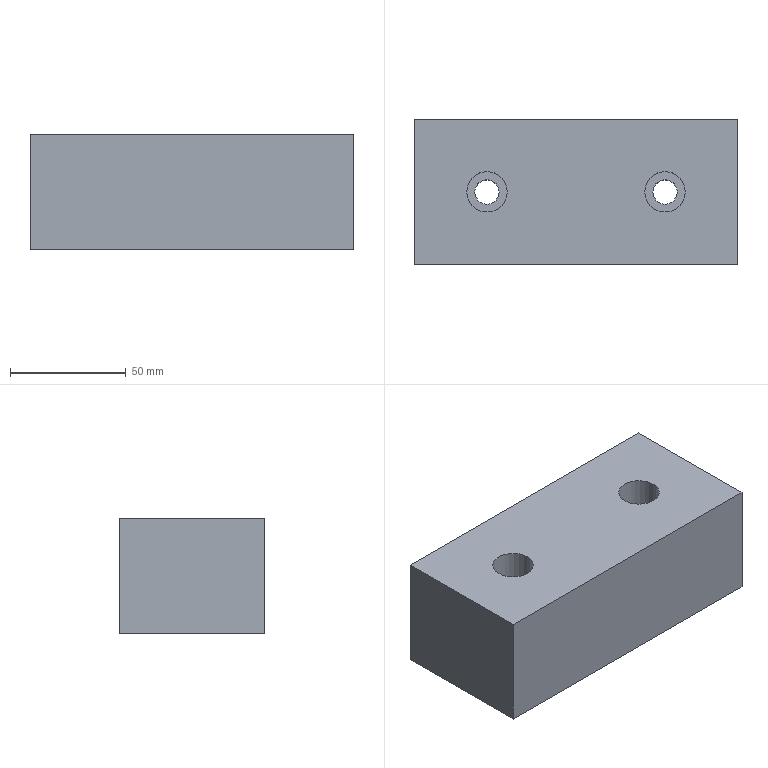Part | NX | features MAIN_BODY 2 | 1 solid | 12 faces | box 140 x 63 x 50 mm | volume 423105 mm3 | plane 8 | cylinder 4 | commonest cylinder face diameters 10.5 x2 17.5 x2
STEP:
#1=CARTESIAN_POINT('',(1506.25,487.5,70.));
#2=VERTEX_POINT('',#1);
#3=CARTESIAN_POINT('',(1511.5,487.5,70.));
#4=DIRECTION('',(0.,0.,-1.));
#5=DIRECTION('',(-1.,0.,0.));
#6=AXIS2_PLACEMENT_3D('',#3,#4,#5);
#7=CIRCLE('',#6,5.25);
#8=EDGE_CURVE('',#2,#2,#7,.F.);
#9=ORIENTED_EDGE('',*,*,#8,.F.);
#10=EDGE_LOOP('',(#9));
#11=FACE_BOUND('',#10,.T.);
#12=CARTESIAN_POINT('',(1506.25,487.5,90.));
#13=VERTEX_POINT('',#12);
#14=CARTESIAN_POINT('',(1511.5,487.5,90.));
#15=DIRECTION('',(0.,0.,-1.));
#16=DIRECTION('',(-1.,0.,0.));
#17=AXIS2_PLACEMENT_3D('',#14,#15,#16);
#18=CIRCLE('',#17,5.25);
#19=EDGE_CURVE('',#13,#13,#18,.F.);
#20=ORIENTED_EDGE('',*,*,#19,.T.);
#21=EDGE_LOOP('',(#20));
#22=FACE_BOUND('',#21,.T.);
#23=CARTESIAN_POINT('',(1511.5,487.5,90.));
#24=DIRECTION('',(0.,0.,-1.));
#25=DIRECTION('',(-1.,0.,0.));
#26=AXIS2_PLACEMENT_3D('',#23,#24,#25);
#27=CYLINDRICAL_SURFACE('',#26,5.25);
#28=ADVANCED_FACE('',(#11,#22),#27,.F.);
#29=CARTESIAN_POINT('',(1593.75,487.5,70.));
#30=VERTEX_POINT('',#29);
#31=CARTESIAN_POINT('',(1588.5,487.5,70.));
#32=DIRECTION('',(0.,0.,1.));
#33=DIRECTION('',(1.,0.,0.));
#34=AXIS2_PLACEMENT_3D('',#31,#32,#33);
#35=CIRCLE('',#34,5.25);
#36=EDGE_CURVE('',#30,#30,#35,.F.);
#37=ORIENTED_EDGE('',*,*,#36,.T.);
#38=EDGE_LOOP('',(#37));
#39=FACE_BOUND('',#38,.T.);
#40=CARTESIAN_POINT('',(1593.75,487.5,90.));
#41=VERTEX_POINT('',#40);
#42=CARTESIAN_POINT('',(1588.5,487.5,90.));
#43=DIRECTION('',(0.,0.,1.));
#44=DIRECTION('',(1.,0.,0.));
#45=AXIS2_PLACEMENT_3D('',#42,#43,#44);
#46=CIRCLE('',#45,5.25);
#47=EDGE_CURVE('',#41,#41,#46,.F.);
#48=ORIENTED_EDGE('',*,*,#47,.F.);
#49=EDGE_LOOP('',(#48));
#50=FACE_BOUND('',#49,.T.);
#51=CARTESIAN_POINT('',(1588.5,487.5,90.));
#52=DIRECTION('',(0.,0.,-1.));
#53=DIRECTION('',(1.,0.,0.));
#54=AXIS2_PLACEMENT_3D('',#51,#52,#53);
#55=CYLINDRICAL_SURFACE('',#54,5.25);
#56=ADVANCED_FACE('',(#39,#50),#55,.F.);
#57=ORIENTED_EDGE('',*,*,#47,.T.);
#58=EDGE_LOOP('',(#57));
#59=FACE_BOUND('',#58,.T.);
#60=CARTESIAN_POINT('',(1597.25,487.5,90.));
#61=VERTEX_POINT('',#60);
#62=CARTESIAN_POINT('',(1588.5,487.5,90.));
#63=DIRECTION('',(0.,0.,-1.));
#64=DIRECTION('',(1.,0.,0.));
#65=AXIS2_PLACEMENT_3D('',#62,#63,#64);
#66=CIRCLE('',#65,8.75);
#67=EDGE_CURVE('',#61,#61,#66,.T.);
#68=ORIENTED_EDGE('',*,*,#67,.F.);
#69=EDGE_LOOP('',(#68));
#70=FACE_BOUND('',#69,.T.);
#71=CARTESIAN_POINT('',(1588.5,487.5,90.));
#72=DIRECTION('',(0.,0.,-1.));
#73=DIRECTION('',(1.,0.,0.));
#74=AXIS2_PLACEMENT_3D('',#71,#72,#73);
#75=PLANE('',#74);
#76=ADVANCED_FACE('',(#59,#70),#75,.F.);
#77=ORIENTED_EDGE('',*,*,#67,.T.);
#78=EDGE_LOOP('',(#77));
#79=FACE_BOUND('',#78,.T.);
#80=CARTESIAN_POINT('',(1597.25,487.5,120.));
#81=VERTEX_POINT('',#80);
#82=CARTESIAN_POINT('',(1588.5,487.5,120.));
#83=DIRECTION('',(0.,0.,1.));
#84=DIRECTION('',(1.,0.,0.));
#85=AXIS2_PLACEMENT_3D('',#82,#83,#84);
#86=CIRCLE('',#85,8.75);
#87=EDGE_CURVE('',#81,#81,#86,.F.);
#88=ORIENTED_EDGE('',*,*,#87,.F.);
#89=EDGE_LOOP('',(#88));
#90=FACE_BOUND('',#89,.T.);
#91=CARTESIAN_POINT('',(1588.5,487.5,70.));
#92=DIRECTION('',(0.,0.,1.));
#93=DIRECTION('',(1.,0.,0.));
#94=AXIS2_PLACEMENT_3D('',#91,#92,#93);
#95=CYLINDRICAL_SURFACE('',#94,8.75);
#96=ADVANCED_FACE('',(#79,#90),#95,.F.);
#97=ORIENTED_EDGE('',*,*,#36,.F.);
#98=EDGE_LOOP('',(#97));
#99=FACE_BOUND('',#98,.T.);
#100=CARTESIAN_POINT('',(1620.,456.,70.));
#101=VERTEX_POINT('',#100);
#102=CARTESIAN_POINT('',(1620.,519.,70.));
#103=VERTEX_POINT('',#102);
#104=CARTESIAN_POINT('',(1620.,469.,70.));
#105=DIRECTION('',(0.,1.,0.));
#106=VECTOR('',#105,1000.);
#107=LINE('',#104,#106);
#108=EDGE_CURVE('',#101,#103,#107,.T.);
#109=ORIENTED_EDGE('',*,*,#108,.F.);
#110=CARTESIAN_POINT('',(1480.,456.,70.));
#111=VERTEX_POINT('',#110);
#112=CARTESIAN_POINT('',(1343.352,456.,70.));
#113=DIRECTION('',(1.,0.,0.));
#114=VECTOR('',#113,1000.);
#115=LINE('',#112,#114);
#116=EDGE_CURVE('',#111,#101,#115,.T.);
#117=ORIENTED_EDGE('',*,*,#116,.F.);
#118=CARTESIAN_POINT('',(1480.,519.,70.));
#119=VERTEX_POINT('',#118);
#120=CARTESIAN_POINT('',(1480.,469.,70.));
#121=DIRECTION('',(0.,1.,0.));
#122=VECTOR('',#121,1000.);
#123=LINE('',#120,#122);
#124=EDGE_CURVE('',#111,#119,#123,.T.);
#125=ORIENTED_EDGE('',*,*,#124,.T.);
#126=CARTESIAN_POINT('',(1343.352,519.,70.));
#127=DIRECTION('',(1.,0.,0.));
#128=VECTOR('',#127,1000.);
#129=LINE('',#126,#128);
#130=EDGE_CURVE('',#119,#103,#129,.T.);
#131=ORIENTED_EDGE('',*,*,#130,.T.);
#132=EDGE_LOOP('',(#109,#117,#125,#131));
#133=FACE_BOUND('',#132,.T.);
#134=ORIENTED_EDGE('',*,*,#8,.T.);
#135=EDGE_LOOP('',(#134));
#136=FACE_BOUND('',#135,.T.);
#137=CARTESIAN_POINT('',(1343.352,469.,70.));
#138=DIRECTION('',(0.,0.,-1.));
#139=DIRECTION('',(-1.,0.,0.));
#140=AXIS2_PLACEMENT_3D('',#137,#138,#139);
#141=PLANE('',#140);
#142=ADVANCED_FACE('',(#99,#133,#136),#141,.T.);
#143=ORIENTED_EDGE('',*,*,#19,.F.);
#144=EDGE_LOOP('',(#143));
#145=FACE_BOUND('',#144,.T.);
#146=CARTESIAN_POINT('',(1502.75,487.5,90.));
#147=VERTEX_POINT('',#146);
#148=CARTESIAN_POINT('',(1511.5,487.5,90.));
#149=DIRECTION('',(0.,0.,1.));
#150=DIRECTION('',(-1.,0.,0.));
#151=AXIS2_PLACEMENT_3D('',#148,#149,#150);
#152=CIRCLE('',#151,8.75);
#153=EDGE_CURVE('',#147,#147,#152,.T.);
#154=ORIENTED_EDGE('',*,*,#153,.T.);
#155=EDGE_LOOP('',(#154));
#156=FACE_BOUND('',#155,.T.);
#157=CARTESIAN_POINT('',(1511.5,487.5,90.));
#158=DIRECTION('',(0.,0.,-1.));
#159=DIRECTION('',(-1.,0.,0.));
#160=AXIS2_PLACEMENT_3D('',#157,#158,#159);
#161=PLANE('',#160);
#162=ADVANCED_FACE('',(#145,#156),#161,.F.);
#163=CARTESIAN_POINT('',(1620.,519.,120.));
#164=VERTEX_POINT('',#163);
#165=CARTESIAN_POINT('',(1620.,456.,120.));
#166=VERTEX_POINT('',#165);
#167=CARTESIAN_POINT('',(1620.,469.,120.));
#168=DIRECTION('',(0.,-1.,0.));
#169=VECTOR('',#168,1000.);
#170=LINE('',#167,#169);
#171=EDGE_CURVE('',#164,#166,#170,.T.);
#172=ORIENTED_EDGE('',*,*,#171,.T.);
#173=CARTESIAN_POINT('',(1620.,456.,228.412));
#174=DIRECTION('',(0.,0.,1.));
#175=VECTOR('',#174,1000.);
#176=LINE('',#173,#175);
#177=EDGE_CURVE('',#101,#166,#176,.T.);
#178=ORIENTED_EDGE('',*,*,#177,.F.);
#179=ORIENTED_EDGE('',*,*,#108,.T.);
#180=CARTESIAN_POINT('',(1620.,519.,70.));
#181=DIRECTION('',(0.,0.,1.));
#182=VECTOR('',#181,1000.);
#183=LINE('',#180,#182);
#184=EDGE_CURVE('',#103,#164,#183,.T.);
#185=ORIENTED_EDGE('',*,*,#184,.T.);
#186=EDGE_LOOP('',(#172,#178,#179,#185));
#187=FACE_BOUND('',#186,.T.);
#188=CARTESIAN_POINT('',(1620.,469.,70.));
#189=DIRECTION('',(1.,0.,0.));
#190=DIRECTION('',(0.,-1.,0.));
#191=AXIS2_PLACEMENT_3D('',#188,#189,#190);
#192=PLANE('',#191);
#193=ADVANCED_FACE('',(#187),#192,.T.);
#194=CARTESIAN_POINT('',(1480.,519.,120.));
#195=VERTEX_POINT('',#194);
#196=CARTESIAN_POINT('',(1480.,456.,120.));
#197=VERTEX_POINT('',#196);
#198=CARTESIAN_POINT('',(1480.,469.,120.));
#199=DIRECTION('',(0.,-1.,0.));
#200=VECTOR('',#199,1000.);
#201=LINE('',#198,#200);
#202=EDGE_CURVE('',#195,#197,#201,.T.);
#203=ORIENTED_EDGE('',*,*,#202,.F.);
#204=CARTESIAN_POINT('',(1480.,519.,70.));
#205=DIRECTION('',(0.,0.,1.));
#206=VECTOR('',#205,1000.);
#207=LINE('',#204,#206);
#208=EDGE_CURVE('',#119,#195,#207,.T.);
#209=ORIENTED_EDGE('',*,*,#208,.F.);
#210=ORIENTED_EDGE('',*,*,#124,.F.);
#211=CARTESIAN_POINT('',(1480.,456.,228.412));
#212=DIRECTION('',(0.,0.,1.));
#213=VECTOR('',#212,1000.);
#214=LINE('',#211,#213);
#215=EDGE_CURVE('',#111,#197,#214,.T.);
#216=ORIENTED_EDGE('',*,*,#215,.T.);
#217=EDGE_LOOP('',(#203,#209,#210,#216));
#218=FACE_BOUND('',#217,.T.);
#219=CARTESIAN_POINT('',(1480.,469.,70.));
#220=DIRECTION('',(-1.,0.,0.));
#221=DIRECTION('',(0.,-1.,0.));
#222=AXIS2_PLACEMENT_3D('',#219,#220,#221);
#223=PLANE('',#222);
#224=ADVANCED_FACE('',(#218),#223,.T.);
#225=ORIENTED_EDGE('',*,*,#171,.F.);
#226=CARTESIAN_POINT('',(1343.352,519.,120.));
#227=DIRECTION('',(1.,0.,0.));
#228=VECTOR('',#227,1000.);
#229=LINE('',#226,#228);
#230=EDGE_CURVE('',#195,#164,#229,.T.);
#231=ORIENTED_EDGE('',*,*,#230,.F.);
#232=ORIENTED_EDGE('',*,*,#202,.T.);
#233=CARTESIAN_POINT('',(1343.352,456.,120.));
#234=DIRECTION('',(1.,0.,0.));
#235=VECTOR('',#234,1000.);
#236=LINE('',#233,#235);
#237=EDGE_CURVE('',#197,#166,#236,.T.);
#238=ORIENTED_EDGE('',*,*,#237,.T.);
#239=EDGE_LOOP('',(#225,#231,#232,#238));
#240=FACE_BOUND('',#239,.T.);
#241=CARTESIAN_POINT('',(1502.75,487.5,120.));
#242=VERTEX_POINT('',#241);
#243=CARTESIAN_POINT('',(1511.5,487.5,120.));
#244=DIRECTION('',(0.,0.,-1.));
#245=DIRECTION('',(-1.,0.,0.));
#246=AXIS2_PLACEMENT_3D('',#243,#244,#245);
#247=CIRCLE('',#246,8.75);
#248=EDGE_CURVE('',#242,#242,#247,.F.);
#249=ORIENTED_EDGE('',*,*,#248,.F.);
#250=EDGE_LOOP('',(#249));
#251=FACE_BOUND('',#250,.T.);
#252=ORIENTED_EDGE('',*,*,#87,.T.);
#253=EDGE_LOOP('',(#252));
#254=FACE_BOUND('',#253,.T.);
#255=CARTESIAN_POINT('',(1550.,487.5,120.));
#256=DIRECTION('',(0.,0.,-1.));
#257=DIRECTION('',(1.,0.,0.));
#258=AXIS2_PLACEMENT_3D('',#255,#256,#257);
#259=PLANE('',#258);
#260=ADVANCED_FACE('',(#240,#251,#254),#259,.F.);
#261=ORIENTED_EDGE('',*,*,#116,.T.);
#262=ORIENTED_EDGE('',*,*,#177,.T.);
#263=ORIENTED_EDGE('',*,*,#237,.F.);
#264=ORIENTED_EDGE('',*,*,#215,.F.);
#265=EDGE_LOOP('',(#261,#262,#263,#264));
#266=FACE_BOUND('',#265,.T.);
#267=CARTESIAN_POINT('',(1343.352,456.,228.412));
#268=DIRECTION('',(0.,1.,0.));
#269=DIRECTION('',(1.,0.,0.));
#270=AXIS2_PLACEMENT_3D('',#267,#268,#269);
#271=PLANE('',#270);
#272=ADVANCED_FACE('',(#266),#271,.F.);
#273=ORIENTED_EDGE('',*,*,#230,.T.);
#274=ORIENTED_EDGE('',*,*,#184,.F.);
#275=ORIENTED_EDGE('',*,*,#130,.F.);
#276=ORIENTED_EDGE('',*,*,#208,.T.);
#277=EDGE_LOOP('',(#273,#274,#275,#276));
#278=FACE_BOUND('',#277,.T.);
#279=CARTESIAN_POINT('',(1343.352,519.,228.412));
#280=DIRECTION('',(0.,1.,0.));
#281=DIRECTION('',(1.,0.,0.));
#282=AXIS2_PLACEMENT_3D('',#279,#280,#281);
#283=PLANE('',#282);
#284=ADVANCED_FACE('',(#278),#283,.T.);
#285=ORIENTED_EDGE('',*,*,#153,.F.);
#286=EDGE_LOOP('',(#285));
#287=FACE_BOUND('',#286,.T.);
#288=ORIENTED_EDGE('',*,*,#248,.T.);
#289=EDGE_LOOP('',(#288));
#290=FACE_BOUND('',#289,.T.);
#291=CARTESIAN_POINT('',(1511.5,487.5,70.));
#292=DIRECTION('',(0.,0.,1.));
#293=DIRECTION('',(-1.,0.,0.));
#294=AXIS2_PLACEMENT_3D('',#291,#292,#293);
#295=CYLINDRICAL_SURFACE('',#294,8.75);
#296=ADVANCED_FACE('',(#287,#290),#295,.F.);
#297=CLOSED_SHELL('',(#28,#56,#76,#96,#142,#162,#193,#224,#260,#272,#284,#296));
#298=MANIFOLD_SOLID_BREP('',#297);
#299=(LENGTH_UNIT()NAMED_UNIT(*)SI_UNIT(.MILLI.,.METRE.));
#300=UNCERTAINTY_MEASURE_WITH_UNIT(LENGTH_MEASURE(0.00001),#299,'','');
#301=(NAMED_UNIT(*)PLANE_ANGLE_UNIT()SI_UNIT($,.RADIAN.));
#302=(NAMED_UNIT(*)SI_UNIT($,.STERADIAN.)SOLID_ANGLE_UNIT());
#303=(GEOMETRIC_REPRESENTATION_CONTEXT(3)GLOBAL_UNCERTAINTY_ASSIGNED_CONTEXT((#300))GLOBAL_UNIT_ASSIGNED_CONTEXT((#299,#301,#302))REPRESENTATION_CONTEXT('',''));
#304=ADVANCED_BREP_SHAPE_REPRESENTATION('',(#298),#303);